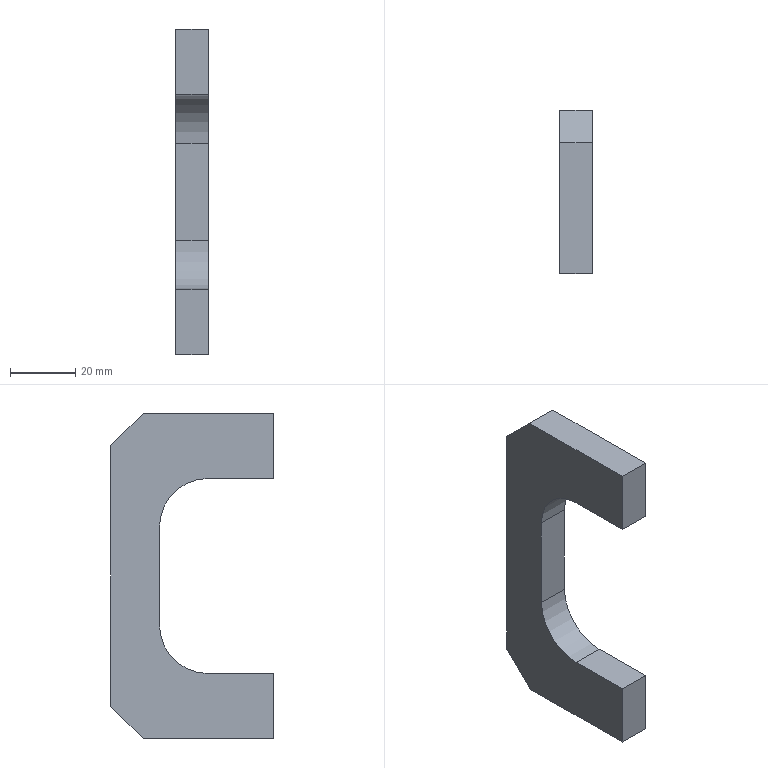Part | STEP file | VD-SYL0380DJ1006_1_2_1-4_STEP | 1 solid | 14 faces | box 10 x 50 x 100 mm | volume 28966 mm3 | plane 12 | cylinder 2 | commonest cylinder face diameters 30 x2
STEP:
#1=CARTESIAN_POINT('',(10.,35.,-15.));
#2=VERTEX_POINT('',#1);
#3=CARTESIAN_POINT('',(10.,35.,15.));
#4=VERTEX_POINT('',#3);
#5=CARTESIAN_POINT('',(10.,35.,-15.));
#6=DIRECTION('',(0.,0.,1.));
#7=VECTOR('',#6,1000.);
#8=LINE('',#5,#7);
#9=EDGE_CURVE('',#2,#4,#8,.T.);
#10=ORIENTED_EDGE('',*,*,#9,.T.);
#11=CARTESIAN_POINT('',(0.,35.,15.));
#12=VERTEX_POINT('',#11);
#13=CARTESIAN_POINT('',(0.,35.,15.));
#14=DIRECTION('',(1.,0.,0.));
#15=VECTOR('',#14,1000.);
#16=LINE('',#13,#15);
#17=EDGE_CURVE('',#12,#4,#16,.T.);
#18=ORIENTED_EDGE('',*,*,#17,.F.);
#19=CARTESIAN_POINT('',(0.,35.,-15.));
#20=VERTEX_POINT('',#19);
#21=CARTESIAN_POINT('',(0.,35.,-15.));
#22=DIRECTION('',(0.,0.,1.));
#23=VECTOR('',#22,1000.);
#24=LINE('',#21,#23);
#25=EDGE_CURVE('',#20,#12,#24,.T.);
#26=ORIENTED_EDGE('',*,*,#25,.F.);
#27=CARTESIAN_POINT('',(10.,35.,-15.));
#28=DIRECTION('',(-1.,0.,0.));
#29=VECTOR('',#28,1000.);
#30=LINE('',#27,#29);
#31=EDGE_CURVE('',#2,#20,#30,.T.);
#32=ORIENTED_EDGE('',*,*,#31,.F.);
#33=EDGE_LOOP('',(#10,#18,#26,#32));
#34=FACE_OUTER_BOUND('',#33,.T.);
#35=CARTESIAN_POINT('',(10.,35.,-30.));
#36=DIRECTION('',(0.,1.,0.));
#37=DIRECTION('',(1.,0.,0.));
#38=AXIS2_PLACEMENT_3D('',#35,#36,#37);
#39=PLANE('',#38);
#40=ADVANCED_FACE('',(#34),#39,.F.);
#41=CARTESIAN_POINT('',(10.,20.,30.));
#42=VERTEX_POINT('',#41);
#43=CARTESIAN_POINT('',(10.,20.,15.));
#44=DIRECTION('',(-1.,0.,0.));
#45=DIRECTION('',(0.,0.,1.));
#46=AXIS2_PLACEMENT_3D('',#43,#44,#45);
#47=CIRCLE('',#46,15.);
#48=EDGE_CURVE('',#42,#4,#47,.T.);
#49=ORIENTED_EDGE('',*,*,#48,.F.);
#50=CARTESIAN_POINT('',(0.,20.,30.));
#51=VERTEX_POINT('',#50);
#52=CARTESIAN_POINT('',(10.,20.,30.));
#53=DIRECTION('',(-1.,0.,0.));
#54=VECTOR('',#53,1000.);
#55=LINE('',#52,#54);
#56=EDGE_CURVE('',#42,#51,#55,.T.);
#57=ORIENTED_EDGE('',*,*,#56,.T.);
#58=CARTESIAN_POINT('',(0.,20.,15.));
#59=DIRECTION('',(1.,0.,0.));
#60=DIRECTION('',(0.,1.,0.));
#61=AXIS2_PLACEMENT_3D('',#58,#59,#60);
#62=CIRCLE('',#61,15.);
#63=EDGE_CURVE('',#12,#51,#62,.T.);
#64=ORIENTED_EDGE('',*,*,#63,.F.);
#65=ORIENTED_EDGE('',*,*,#17,.T.);
#66=EDGE_LOOP('',(#49,#57,#64,#65));
#67=FACE_OUTER_BOUND('',#66,.T.);
#68=CARTESIAN_POINT('',(29.048,20.,15.));
#69=DIRECTION('',(-1.,0.,0.));
#70=DIRECTION('',(0.,0.,1.));
#71=AXIS2_PLACEMENT_3D('',#68,#69,#70);
#72=CYLINDRICAL_SURFACE('',#71,15.);
#73=ADVANCED_FACE('',(#67),#72,.F.);
#74=CARTESIAN_POINT('',(0.,40.,50.));
#75=VERTEX_POINT('',#74);
#76=CARTESIAN_POINT('',(0.,50.,40.));
#77=VERTEX_POINT('',#76);
#78=CARTESIAN_POINT('',(0.,40.,50.));
#79=DIRECTION('',(0.,0.7071,-0.7071));
#80=VECTOR('',#79,1000.);
#81=LINE('',#78,#80);
#82=EDGE_CURVE('',#75,#77,#81,.T.);
#83=ORIENTED_EDGE('',*,*,#82,.F.);
#84=CARTESIAN_POINT('',(10.,40.,50.));
#85=VERTEX_POINT('',#84);
#86=CARTESIAN_POINT('',(0.,40.,50.));
#87=DIRECTION('',(1.,0.,0.));
#88=VECTOR('',#87,1000.);
#89=LINE('',#86,#88);
#90=EDGE_CURVE('',#75,#85,#89,.T.);
#91=ORIENTED_EDGE('',*,*,#90,.T.);
#92=CARTESIAN_POINT('',(10.,50.,40.));
#93=VERTEX_POINT('',#92);
#94=CARTESIAN_POINT('',(10.,50.,40.));
#95=DIRECTION('',(0.,-0.7071,0.7071));
#96=VECTOR('',#95,1000.);
#97=LINE('',#94,#96);
#98=EDGE_CURVE('',#93,#85,#97,.T.);
#99=ORIENTED_EDGE('',*,*,#98,.F.);
#100=CARTESIAN_POINT('',(0.,50.,40.));
#101=DIRECTION('',(1.,0.,0.));
#102=VECTOR('',#101,1000.);
#103=LINE('',#100,#102);
#104=EDGE_CURVE('',#77,#93,#103,.T.);
#105=ORIENTED_EDGE('',*,*,#104,.F.);
#106=EDGE_LOOP('',(#83,#91,#99,#105));
#107=FACE_OUTER_BOUND('',#106,.T.);
#108=CARTESIAN_POINT('',(0.,50.,40.));
#109=DIRECTION('',(0.,0.7071,0.7071));
#110=DIRECTION('',(1.,0.,0.));
#111=AXIS2_PLACEMENT_3D('',#108,#109,#110);
#112=PLANE('',#111);
#113=ADVANCED_FACE('',(#107),#112,.T.);
#114=CARTESIAN_POINT('',(0.,0.,50.));
#115=VERTEX_POINT('',#114);
#116=CARTESIAN_POINT('',(0.,0.,50.));
#117=DIRECTION('',(0.,1.,0.));
#118=VECTOR('',#117,1000.);
#119=LINE('',#116,#118);
#120=EDGE_CURVE('',#115,#75,#119,.T.);
#121=ORIENTED_EDGE('',*,*,#120,.F.);
#122=CARTESIAN_POINT('',(10.,0.,50.));
#123=VERTEX_POINT('',#122);
#124=CARTESIAN_POINT('',(0.,0.,50.));
#125=DIRECTION('',(1.,0.,0.));
#126=VECTOR('',#125,1000.);
#127=LINE('',#124,#126);
#128=EDGE_CURVE('',#115,#123,#127,.T.);
#129=ORIENTED_EDGE('',*,*,#128,.T.);
#130=CARTESIAN_POINT('',(10.,40.,50.));
#131=DIRECTION('',(0.,-1.,0.));
#132=VECTOR('',#131,1000.);
#133=LINE('',#130,#132);
#134=EDGE_CURVE('',#85,#123,#133,.T.);
#135=ORIENTED_EDGE('',*,*,#134,.F.);
#136=ORIENTED_EDGE('',*,*,#90,.F.);
#137=EDGE_LOOP('',(#121,#129,#135,#136));
#138=FACE_OUTER_BOUND('',#137,.T.);
#139=CARTESIAN_POINT('',(0.,40.,50.));
#140=DIRECTION('',(0.,0.,1.));
#141=DIRECTION('',(1.,0.,0.));
#142=AXIS2_PLACEMENT_3D('',#139,#140,#141);
#143=PLANE('',#142);
#144=ADVANCED_FACE('',(#138),#143,.T.);
#145=CARTESIAN_POINT('',(10.,0.,30.));
#146=VERTEX_POINT('',#145);
#147=CARTESIAN_POINT('',(0.,0.,30.));
#148=VERTEX_POINT('',#147);
#149=CARTESIAN_POINT('',(10.,0.,30.));
#150=DIRECTION('',(-1.,0.,0.));
#151=VECTOR('',#150,1000.);
#152=LINE('',#149,#151);
#153=EDGE_CURVE('',#146,#148,#152,.T.);
#154=ORIENTED_EDGE('',*,*,#153,.F.);
#155=CARTESIAN_POINT('',(10.,0.,50.));
#156=DIRECTION('',(0.,0.,-1.));
#157=VECTOR('',#156,1000.);
#158=LINE('',#155,#157);
#159=EDGE_CURVE('',#123,#146,#158,.T.);
#160=ORIENTED_EDGE('',*,*,#159,.F.);
#161=ORIENTED_EDGE('',*,*,#128,.F.);
#162=CARTESIAN_POINT('',(0.,0.,30.));
#163=DIRECTION('',(0.,0.,1.));
#164=VECTOR('',#163,1000.);
#165=LINE('',#162,#164);
#166=EDGE_CURVE('',#148,#115,#165,.T.);
#167=ORIENTED_EDGE('',*,*,#166,.F.);
#168=EDGE_LOOP('',(#154,#160,#161,#167));
#169=FACE_OUTER_BOUND('',#168,.T.);
#170=CARTESIAN_POINT('',(0.,0.,50.));
#171=DIRECTION('',(0.,-1.,0.));
#172=DIRECTION('',(0.,0.,-1.));
#173=AXIS2_PLACEMENT_3D('',#170,#171,#172);
#174=PLANE('',#173);
#175=ADVANCED_FACE('',(#169),#174,.T.);
#176=CARTESIAN_POINT('',(0.,20.,30.));
#177=DIRECTION('',(0.,-1.,0.));
#178=VECTOR('',#177,1000.);
#179=LINE('',#176,#178);
#180=EDGE_CURVE('',#51,#148,#179,.T.);
#181=ORIENTED_EDGE('',*,*,#180,.F.);
#182=ORIENTED_EDGE('',*,*,#56,.F.);
#183=CARTESIAN_POINT('',(10.,20.,30.));
#184=DIRECTION('',(0.,-1.,0.));
#185=VECTOR('',#184,1000.);
#186=LINE('',#183,#185);
#187=EDGE_CURVE('',#42,#146,#186,.T.);
#188=ORIENTED_EDGE('',*,*,#187,.T.);
#189=ORIENTED_EDGE('',*,*,#153,.T.);
#190=EDGE_LOOP('',(#181,#182,#188,#189));
#191=FACE_OUTER_BOUND('',#190,.T.);
#192=CARTESIAN_POINT('',(10.,35.,30.));
#193=DIRECTION('',(0.,0.,1.));
#194=DIRECTION('',(1.,0.,0.));
#195=AXIS2_PLACEMENT_3D('',#192,#193,#194);
#196=PLANE('',#195);
#197=ADVANCED_FACE('',(#191),#196,.F.);
#198=ORIENTED_EDGE('',*,*,#166,.T.);
#199=ORIENTED_EDGE('',*,*,#120,.T.);
#200=ORIENTED_EDGE('',*,*,#82,.T.);
#201=CARTESIAN_POINT('',(0.,50.,-40.));
#202=VERTEX_POINT('',#201);
#203=CARTESIAN_POINT('',(0.,50.,40.));
#204=DIRECTION('',(0.,0.,-1.));
#205=VECTOR('',#204,1000.);
#206=LINE('',#203,#205);
#207=EDGE_CURVE('',#77,#202,#206,.T.);
#208=ORIENTED_EDGE('',*,*,#207,.T.);
#209=CARTESIAN_POINT('',(0.,40.,-50.));
#210=VERTEX_POINT('',#209);
#211=CARTESIAN_POINT('',(0.,50.,-40.));
#212=DIRECTION('',(0.,-0.7071,-0.7071));
#213=VECTOR('',#212,1000.);
#214=LINE('',#211,#213);
#215=EDGE_CURVE('',#202,#210,#214,.T.);
#216=ORIENTED_EDGE('',*,*,#215,.T.);
#217=CARTESIAN_POINT('',(0.,0.,-50.));
#218=VERTEX_POINT('',#217);
#219=CARTESIAN_POINT('',(0.,40.,-50.));
#220=DIRECTION('',(0.,-1.,0.));
#221=VECTOR('',#220,1000.);
#222=LINE('',#219,#221);
#223=EDGE_CURVE('',#210,#218,#222,.T.);
#224=ORIENTED_EDGE('',*,*,#223,.T.);
#225=CARTESIAN_POINT('',(0.,0.,-30.));
#226=VERTEX_POINT('',#225);
#227=CARTESIAN_POINT('',(0.,0.,-50.));
#228=DIRECTION('',(0.,0.,1.));
#229=VECTOR('',#228,1000.);
#230=LINE('',#227,#229);
#231=EDGE_CURVE('',#218,#226,#230,.T.);
#232=ORIENTED_EDGE('',*,*,#231,.T.);
#233=CARTESIAN_POINT('',(0.,20.,-30.));
#234=VERTEX_POINT('',#233);
#235=CARTESIAN_POINT('',(0.,0.,-30.));
#236=DIRECTION('',(0.,1.,0.));
#237=VECTOR('',#236,1000.);
#238=LINE('',#235,#237);
#239=EDGE_CURVE('',#226,#234,#238,.T.);
#240=ORIENTED_EDGE('',*,*,#239,.T.);
#241=CARTESIAN_POINT('',(0.,20.,-15.));
#242=DIRECTION('',(1.,0.,0.));
#243=DIRECTION('',(0.,0.,-1.));
#244=AXIS2_PLACEMENT_3D('',#241,#242,#243);
#245=CIRCLE('',#244,15.);
#246=EDGE_CURVE('',#234,#20,#245,.T.);
#247=ORIENTED_EDGE('',*,*,#246,.T.);
#248=ORIENTED_EDGE('',*,*,#25,.T.);
#249=ORIENTED_EDGE('',*,*,#63,.T.);
#250=ORIENTED_EDGE('',*,*,#180,.T.);
#251=EDGE_LOOP('',(#198,#199,#200,#208,#216,#224,#232,#240,#247,#248,#249,#250));
#252=FACE_OUTER_BOUND('',#251,.T.);
#253=CARTESIAN_POINT('',(0.,0.,0.));
#254=DIRECTION('',(1.,0.,0.));
#255=DIRECTION('',(0.,1.,0.));
#256=AXIS2_PLACEMENT_3D('',#253,#254,#255);
#257=PLANE('',#256);
#258=ADVANCED_FACE('',(#252),#257,.F.);
#259=CARTESIAN_POINT('',(10.,0.,-30.));
#260=VERTEX_POINT('',#259);
#261=CARTESIAN_POINT('',(10.,20.,-30.));
#262=VERTEX_POINT('',#261);
#263=CARTESIAN_POINT('',(10.,0.,-30.));
#264=DIRECTION('',(0.,1.,0.));
#265=VECTOR('',#264,1000.);
#266=LINE('',#263,#265);
#267=EDGE_CURVE('',#260,#262,#266,.T.);
#268=ORIENTED_EDGE('',*,*,#267,.T.);
#269=CARTESIAN_POINT('',(0.,20.,-30.));
#270=DIRECTION('',(1.,0.,0.));
#271=VECTOR('',#270,1000.);
#272=LINE('',#269,#271);
#273=EDGE_CURVE('',#234,#262,#272,.T.);
#274=ORIENTED_EDGE('',*,*,#273,.F.);
#275=ORIENTED_EDGE('',*,*,#239,.F.);
#276=CARTESIAN_POINT('',(0.,0.,-30.));
#277=DIRECTION('',(1.,0.,0.));
#278=VECTOR('',#277,1000.);
#279=LINE('',#276,#278);
#280=EDGE_CURVE('',#226,#260,#279,.T.);
#281=ORIENTED_EDGE('',*,*,#280,.T.);
#282=EDGE_LOOP('',(#268,#274,#275,#281));
#283=FACE_OUTER_BOUND('',#282,.T.);
#284=CARTESIAN_POINT('',(10.,0.,-30.));
#285=DIRECTION('',(0.,0.,-1.));
#286=DIRECTION('',(0.,-1.,0.));
#287=AXIS2_PLACEMENT_3D('',#284,#285,#286);
#288=PLANE('',#287);
#289=ADVANCED_FACE('',(#283),#288,.F.);
#290=CARTESIAN_POINT('',(10.,20.,-15.));
#291=DIRECTION('',(-1.,0.,0.));
#292=DIRECTION('',(0.,1.,0.));
#293=AXIS2_PLACEMENT_3D('',#290,#291,#292);
#294=CIRCLE('',#293,15.);
#295=EDGE_CURVE('',#2,#262,#294,.T.);
#296=ORIENTED_EDGE('',*,*,#295,.F.);
#297=ORIENTED_EDGE('',*,*,#31,.T.);
#298=ORIENTED_EDGE('',*,*,#246,.F.);
#299=ORIENTED_EDGE('',*,*,#273,.T.);
#300=EDGE_LOOP('',(#296,#297,#298,#299));
#301=FACE_OUTER_BOUND('',#300,.T.);
#302=CARTESIAN_POINT('',(29.048,20.,-15.));
#303=DIRECTION('',(-1.,0.,0.));
#304=DIRECTION('',(0.,0.,1.));
#305=AXIS2_PLACEMENT_3D('',#302,#303,#304);
#306=CYLINDRICAL_SURFACE('',#305,15.);
#307=ADVANCED_FACE('',(#301),#306,.F.);
#308=ORIENTED_EDGE('',*,*,#267,.F.);
#309=CARTESIAN_POINT('',(10.,0.,-50.));
#310=VERTEX_POINT('',#309);
#311=CARTESIAN_POINT('',(10.,0.,-30.));
#312=DIRECTION('',(0.,0.,-1.));
#313=VECTOR('',#312,1000.);
#314=LINE('',#311,#313);
#315=EDGE_CURVE('',#260,#310,#314,.T.);
#316=ORIENTED_EDGE('',*,*,#315,.T.);
#317=CARTESIAN_POINT('',(10.,40.,-50.));
#318=VERTEX_POINT('',#317);
#319=CARTESIAN_POINT('',(10.,0.,-50.));
#320=DIRECTION('',(0.,1.,0.));
#321=VECTOR('',#320,1000.);
#322=LINE('',#319,#321);
#323=EDGE_CURVE('',#310,#318,#322,.T.);
#324=ORIENTED_EDGE('',*,*,#323,.T.);
#325=CARTESIAN_POINT('',(10.,50.,-40.));
#326=VERTEX_POINT('',#325);
#327=CARTESIAN_POINT('',(10.,40.,-50.));
#328=DIRECTION('',(0.,0.7071,0.7071));
#329=VECTOR('',#328,1000.);
#330=LINE('',#327,#329);
#331=EDGE_CURVE('',#318,#326,#330,.T.);
#332=ORIENTED_EDGE('',*,*,#331,.T.);
#333=CARTESIAN_POINT('',(10.,50.,-40.));
#334=DIRECTION('',(0.,0.,1.));
#335=VECTOR('',#334,1000.);
#336=LINE('',#333,#335);
#337=EDGE_CURVE('',#326,#93,#336,.T.);
#338=ORIENTED_EDGE('',*,*,#337,.T.);
#339=ORIENTED_EDGE('',*,*,#98,.T.);
#340=ORIENTED_EDGE('',*,*,#134,.T.);
#341=ORIENTED_EDGE('',*,*,#159,.T.);
#342=ORIENTED_EDGE('',*,*,#187,.F.);
#343=ORIENTED_EDGE('',*,*,#48,.T.);
#344=ORIENTED_EDGE('',*,*,#9,.F.);
#345=ORIENTED_EDGE('',*,*,#295,.T.);
#346=EDGE_LOOP('',(#308,#316,#324,#332,#338,#339,#340,#341,#342,#343,#344,#345));
#347=FACE_OUTER_BOUND('',#346,.T.);
#348=CARTESIAN_POINT('',(10.,0.,0.));
#349=DIRECTION('',(1.,0.,0.));
#350=DIRECTION('',(0.,1.,0.));
#351=AXIS2_PLACEMENT_3D('',#348,#349,#350);
#352=PLANE('',#351);
#353=ADVANCED_FACE('',(#347),#352,.T.);
#354=ORIENTED_EDGE('',*,*,#280,.F.);
#355=ORIENTED_EDGE('',*,*,#231,.F.);
#356=CARTESIAN_POINT('',(0.,0.,-50.));
#357=DIRECTION('',(1.,0.,0.));
#358=VECTOR('',#357,1000.);
#359=LINE('',#356,#358);
#360=EDGE_CURVE('',#218,#310,#359,.T.);
#361=ORIENTED_EDGE('',*,*,#360,.T.);
#362=ORIENTED_EDGE('',*,*,#315,.F.);
#363=EDGE_LOOP('',(#354,#355,#361,#362));
#364=FACE_OUTER_BOUND('',#363,.T.);
#365=CARTESIAN_POINT('',(0.,0.,50.));
#366=DIRECTION('',(0.,-1.,0.));
#367=DIRECTION('',(0.,0.,-1.));
#368=AXIS2_PLACEMENT_3D('',#365,#366,#367);
#369=PLANE('',#368);
#370=ADVANCED_FACE('',(#364),#369,.T.);
#371=ORIENTED_EDGE('',*,*,#223,.F.);
#372=CARTESIAN_POINT('',(0.,40.,-50.));
#373=DIRECTION('',(1.,0.,0.));
#374=VECTOR('',#373,1000.);
#375=LINE('',#372,#374);
#376=EDGE_CURVE('',#210,#318,#375,.T.);
#377=ORIENTED_EDGE('',*,*,#376,.T.);
#378=ORIENTED_EDGE('',*,*,#323,.F.);
#379=ORIENTED_EDGE('',*,*,#360,.F.);
#380=EDGE_LOOP('',(#371,#377,#378,#379));
#381=FACE_OUTER_BOUND('',#380,.T.);
#382=CARTESIAN_POINT('',(0.,0.,-50.));
#383=DIRECTION('',(0.,0.,-1.));
#384=DIRECTION('',(0.,-1.,0.));
#385=AXIS2_PLACEMENT_3D('',#382,#383,#384);
#386=PLANE('',#385);
#387=ADVANCED_FACE('',(#381),#386,.T.);
#388=ORIENTED_EDGE('',*,*,#215,.F.);
#389=CARTESIAN_POINT('',(0.,50.,-40.));
#390=DIRECTION('',(1.,0.,0.));
#391=VECTOR('',#390,1000.);
#392=LINE('',#389,#391);
#393=EDGE_CURVE('',#202,#326,#392,.T.);
#394=ORIENTED_EDGE('',*,*,#393,.T.);
#395=ORIENTED_EDGE('',*,*,#331,.F.);
#396=ORIENTED_EDGE('',*,*,#376,.F.);
#397=EDGE_LOOP('',(#388,#394,#395,#396));
#398=FACE_OUTER_BOUND('',#397,.T.);
#399=CARTESIAN_POINT('',(0.,40.,-50.));
#400=DIRECTION('',(0.,0.7071,-0.7071));
#401=DIRECTION('',(-1.,0.,0.));
#402=AXIS2_PLACEMENT_3D('',#399,#400,#401);
#403=PLANE('',#402);
#404=ADVANCED_FACE('',(#398),#403,.T.);
#405=ORIENTED_EDGE('',*,*,#207,.F.);
#406=ORIENTED_EDGE('',*,*,#104,.T.);
#407=ORIENTED_EDGE('',*,*,#337,.F.);
#408=ORIENTED_EDGE('',*,*,#393,.F.);
#409=EDGE_LOOP('',(#405,#406,#407,#408));
#410=FACE_OUTER_BOUND('',#409,.T.);
#411=CARTESIAN_POINT('',(0.,50.,-40.));
#412=DIRECTION('',(0.,1.,0.));
#413=DIRECTION('',(1.,0.,0.));
#414=AXIS2_PLACEMENT_3D('',#411,#412,#413);
#415=PLANE('',#414);
#416=ADVANCED_FACE('',(#410),#415,.T.);
#417=CLOSED_SHELL('',(#40,#73,#113,#144,#175,#197,#258,#289,#307,#353,#370,#387,#404,#416));
#418=MANIFOLD_SOLID_BREP('',#417);
#419=CARTESIAN_POINT('',(0.,0.,0.));
#420=DIRECTION('',(0.,0.,1.));
#421=DIRECTION('',(1.,0.,0.));
#422=AXIS2_PLACEMENT_3D('',#419,#420,#421);
#423=(LENGTH_UNIT()NAMED_UNIT(*)SI_UNIT(.MILLI.,.METRE.));
#424=UNCERTAINTY_MEASURE_WITH_UNIT(LENGTH_MEASURE(0.00001),#423,'','');
#425=(NAMED_UNIT(*)PLANE_ANGLE_UNIT()SI_UNIT($,.RADIAN.));
#426=(NAMED_UNIT(*)SI_UNIT($,.STERADIAN.)SOLID_ANGLE_UNIT());
#427=(GEOMETRIC_REPRESENTATION_CONTEXT(3)GLOBAL_UNCERTAINTY_ASSIGNED_CONTEXT((#424))GLOBAL_UNIT_ASSIGNED_CONTEXT((#423,#425,#426))REPRESENTATION_CONTEXT('',''));
#428=ADVANCED_BREP_SHAPE_REPRESENTATION('',(#418,#422),#427);